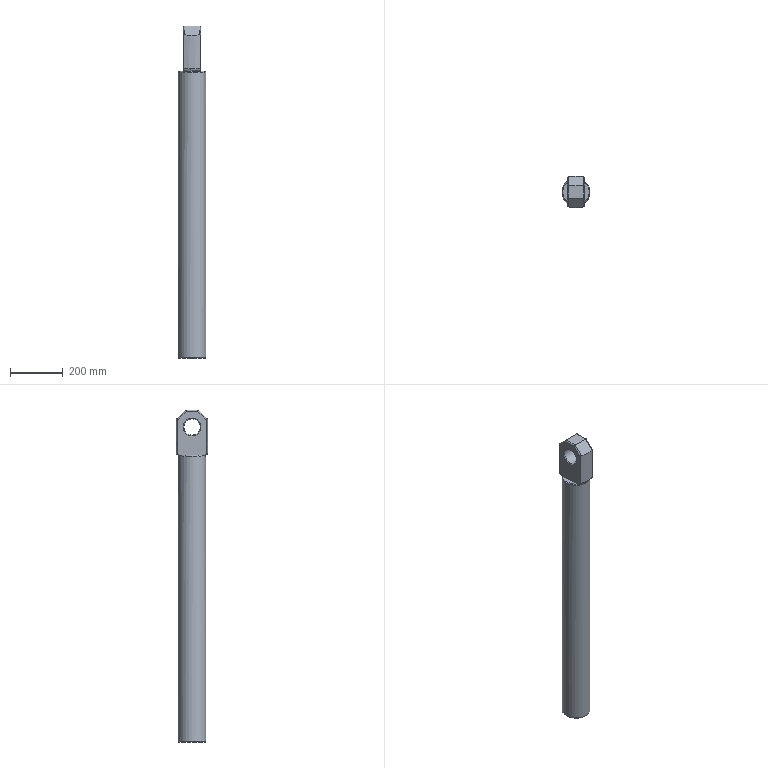Part | NX | features 推移千斤顶活塞 2 | 1 solid | 26 faces | box 106.3 x 120.47 x 1261 mm | volume 10694769 mm3 | cylinder 10 | plane 10 | cone 4 | torus 2 | commonest cylinder face diameters 10 x6 240.94 x2 62 x1 106.3 x1
STEP:
#1=CARTESIAN_POINT('',(-32.42,55.791,1222.469));
#2=VERTEX_POINT('',#1);
#3=CARTESIAN_POINT('',(-32.42,55.791,1099.14));
#4=VERTEX_POINT('',#3);
#5=CARTESIAN_POINT('',(-32.42,55.791,1261.34));
#6=DIRECTION('',(0.,0.,-1.));
#7=VECTOR('',#6,1000.);
#8=LINE('',#5,#7);
#9=EDGE_CURVE('',#2,#4,#8,.T.);
#10=ORIENTED_EDGE('',*,*,#9,.F.);
#11=CARTESIAN_POINT('',(-27.42,57.073,1228.257));
#12=VERTEX_POINT('',#11);
#13=CARTESIAN_POINT('',(-32.42,55.791,1222.469));
#14=CARTESIAN_POINT('',(-32.42,55.791,1223.22));
#15=CARTESIAN_POINT('',(-32.256,55.837,1224.702));
#16=CARTESIAN_POINT('',(-31.381,56.079,1226.805));
#17=CARTESIAN_POINT('',(-29.666,56.532,1228.32));
#18=CARTESIAN_POINT('',(-28.139,56.905,1228.425));
#19=CARTESIAN_POINT('',(-27.42,57.073,1228.257));
#20=B_SPLINE_CURVE_WITH_KNOTS('',3,(#13,#14,#15,#16,#17,#18,#19),.UNSPECIFIED.,.F.,.F.,(4,1,1,1,4),(0.,0.002231,0.004461,0.006692,0.008922),.UNSPECIFIED.);
#21=EDGE_CURVE('',#2,#12,#20,.T.);
#22=ORIENTED_EDGE('',*,*,#21,.T.);
#23=CARTESIAN_POINT('',(27.42,57.073,1228.257));
#24=VERTEX_POINT('',#23);
#25=CARTESIAN_POINT('',(0.,-60.235,1345.565));
#26=DIRECTION('',(0.,0.7071,0.7071));
#27=DIRECTION('',(0.,0.7071,-0.7071));
#28=AXIS2_PLACEMENT_3D('',#25,#26,#27);
#29=ELLIPSE('',#28,170.37,120.47);
#30=EDGE_CURVE('',#24,#12,#29,.T.);
#31=ORIENTED_EDGE('',*,*,#30,.F.);
#32=CARTESIAN_POINT('',(32.42,55.791,1222.469));
#33=VERTEX_POINT('',#32);
#34=CARTESIAN_POINT('',(27.42,57.073,1228.257));
#35=CARTESIAN_POINT('',(28.138,56.905,1228.425));
#36=CARTESIAN_POINT('',(29.654,56.535,1228.326));
#37=CARTESIAN_POINT('',(31.384,56.078,1226.8));
#38=CARTESIAN_POINT('',(32.251,55.838,1224.718));
#39=CARTESIAN_POINT('',(32.42,55.791,1223.22));
#40=CARTESIAN_POINT('',(32.42,55.791,1222.469));
#41=B_SPLINE_CURVE_WITH_KNOTS('',3,(#34,#35,#36,#37,#38,#39,#40),.UNSPECIFIED.,.F.,.F.,(4,1,1,1,4),(0.,0.002239,0.004478,0.006717,0.008957),.UNSPECIFIED.);
#42=EDGE_CURVE('',#24,#33,#41,.T.);
#43=ORIENTED_EDGE('',*,*,#42,.T.);
#44=CARTESIAN_POINT('',(32.42,55.791,1099.14));
#45=VERTEX_POINT('',#44);
#46=CARTESIAN_POINT('',(32.42,55.791,1261.34));
#47=DIRECTION('',(0.,0.,-1.));
#48=VECTOR('',#47,1000.);
#49=LINE('',#46,#48);
#50=EDGE_CURVE('',#33,#45,#49,.T.);
#51=ORIENTED_EDGE('',*,*,#50,.T.);
#52=CARTESIAN_POINT('',(0.,-60.235,1099.14));
#53=DIRECTION('',(0.,0.,1.));
#54=DIRECTION('',(1.,0.,0.));
#55=AXIS2_PLACEMENT_3D('',#52,#53,#54);
#56=CIRCLE('',#55,120.47);
#57=EDGE_CURVE('',#45,#4,#56,.T.);
#58=ORIENTED_EDGE('',*,*,#57,.T.);
#59=EDGE_LOOP('',(#10,#22,#31,#43,#51,#58));
#60=FACE_BOUND('',#59,.T.);
#61=CARTESIAN_POINT('',(0.,-60.235,1261.34));
#62=DIRECTION('',(0.,0.,-1.));
#63=DIRECTION('',(-1.,0.,0.));
#64=AXIS2_PLACEMENT_3D('',#61,#62,#63);
#65=CYLINDRICAL_SURFACE('',#64,120.47);
#66=ADVANCED_FACE('',(#60),#65,.T.);
#67=CARTESIAN_POINT('',(-32.42,34.,1196.49));
#68=VERTEX_POINT('',#67);
#69=CARTESIAN_POINT('',(-32.42,0.,1196.49));
#70=DIRECTION('',(1.,0.,0.));
#71=DIRECTION('',(0.,1.,0.));
#72=AXIS2_PLACEMENT_3D('',#69,#70,#71);
#73=CIRCLE('',#72,34.);
#74=EDGE_CURVE('',#68,#68,#73,.T.);
#75=ORIENTED_EDGE('',*,*,#74,.T.);
#76=EDGE_LOOP('',(#75));
#77=FACE_BOUND('',#76,.T.);
#78=CARTESIAN_POINT('',(-32.42,-21.919,1256.34));
#79=VERTEX_POINT('',#78);
#80=CARTESIAN_POINT('',(-32.42,21.919,1256.34));
#81=VERTEX_POINT('',#80);
#82=CARTESIAN_POINT('',(-32.42,23.99,1256.34));
#83=DIRECTION('',(0.,-1.,0.));
#84=VECTOR('',#83,1000.);
#85=LINE('',#82,#84);
#86=EDGE_CURVE('',#79,#81,#85,.F.);
#87=ORIENTED_EDGE('',*,*,#86,.T.);
#88=CARTESIAN_POINT('',(-32.42,52.255,1226.004));
#89=DIRECTION('',(0.,-0.7071,0.7071));
#90=VECTOR('',#89,1000.);
#91=LINE('',#88,#90);
#92=EDGE_CURVE('',#81,#2,#91,.F.);
#93=ORIENTED_EDGE('',*,*,#92,.T.);
#94=ORIENTED_EDGE('',*,*,#9,.T.);
#95=CARTESIAN_POINT('',(-32.42,45.371,1089.14));
#96=VERTEX_POINT('',#95);
#97=CARTESIAN_POINT('',(-32.42,55.791,1099.14));
#98=CARTESIAN_POINT('',(-32.42,55.791,1096.442));
#99=CARTESIAN_POINT('',(-32.42,53.409,1091.199));
#100=CARTESIAN_POINT('',(-32.42,48.066,1089.14));
#101=CARTESIAN_POINT('',(-32.42,45.371,1089.14));
#102=B_SPLINE_CURVE_WITH_KNOTS('',3,(#97,#98,#99,#100,#101),.UNSPECIFIED.,.F.,.F.,(4,1,4),(0.,0.007978,0.01596),.UNSPECIFIED.);
#103=EDGE_CURVE('',#4,#96,#102,.T.);
#104=ORIENTED_EDGE('',*,*,#103,.T.);
#105=CARTESIAN_POINT('',(-32.42,38.262,1089.14));
#106=VERTEX_POINT('',#105);
#107=CARTESIAN_POINT('',(-32.42,55.791,1089.14));
#108=DIRECTION('',(0.,-1.,0.));
#109=VECTOR('',#108,1000.);
#110=LINE('',#107,#109);
#111=EDGE_CURVE('',#96,#106,#110,.T.);
#112=ORIENTED_EDGE('',*,*,#111,.T.);
#113=CARTESIAN_POINT('',(-32.42,-38.262,1089.14));
#114=VERTEX_POINT('',#113);
#115=CARTESIAN_POINT('',(-32.42,55.791,1089.14));
#116=DIRECTION('',(0.,-1.,0.));
#117=VECTOR('',#116,1000.);
#118=LINE('',#115,#117);
#119=EDGE_CURVE('',#106,#114,#118,.T.);
#120=ORIENTED_EDGE('',*,*,#119,.T.);
#121=CARTESIAN_POINT('',(-32.42,-45.371,1089.14));
#122=VERTEX_POINT('',#121);
#123=CARTESIAN_POINT('',(-32.42,55.791,1089.14));
#124=DIRECTION('',(0.,-1.,0.));
#125=VECTOR('',#124,1000.);
#126=LINE('',#123,#125);
#127=EDGE_CURVE('',#114,#122,#126,.T.);
#128=ORIENTED_EDGE('',*,*,#127,.T.);
#129=CARTESIAN_POINT('',(-32.42,-55.791,1099.14));
#130=VERTEX_POINT('',#129);
#131=CARTESIAN_POINT('',(-32.42,-45.371,1089.14));
#132=CARTESIAN_POINT('',(-32.42,-48.068,1089.14));
#133=CARTESIAN_POINT('',(-32.42,-53.397,1091.189));
#134=CARTESIAN_POINT('',(-32.42,-55.791,1096.44));
#135=CARTESIAN_POINT('',(-32.42,-55.791,1099.14));
#136=B_SPLINE_CURVE_WITH_KNOTS('',3,(#131,#132,#133,#134,#135),.UNSPECIFIED.,.F.,.F.,(4,1,4),(0.,0.007978,0.01596),.UNSPECIFIED.);
#137=EDGE_CURVE('',#122,#130,#136,.T.);
#138=ORIENTED_EDGE('',*,*,#137,.T.);
#139=CARTESIAN_POINT('',(-32.42,-55.791,1222.469));
#140=VERTEX_POINT('',#139);
#141=CARTESIAN_POINT('',(-32.42,-55.791,1261.34));
#142=DIRECTION('',(0.,0.,-1.));
#143=VECTOR('',#142,1000.);
#144=LINE('',#141,#143);
#145=EDGE_CURVE('',#140,#130,#144,.T.);
#146=ORIENTED_EDGE('',*,*,#145,.F.);
#147=CARTESIAN_POINT('',(-32.42,-20.455,1257.804));
#148=DIRECTION('',(0.,-0.7071,-0.7071));
#149=VECTOR('',#148,1000.);
#150=LINE('',#147,#149);
#151=EDGE_CURVE('',#140,#79,#150,.F.);
#152=ORIENTED_EDGE('',*,*,#151,.T.);
#153=EDGE_LOOP('',(#87,#93,#94,#104,#112,#120,#128,#138,#146,#152));
#154=FACE_BOUND('',#153,.T.);
#155=CARTESIAN_POINT('',(-32.42,55.791,1261.34));
#156=DIRECTION('',(1.,0.,0.));
#157=DIRECTION('',(0.,1.,0.));
#158=AXIS2_PLACEMENT_3D('',#155,#156,#157);
#159=PLANE('',#158);
#160=ADVANCED_FACE('',(#77,#154),#159,.F.);
#161=CARTESIAN_POINT('',(-27.42,-57.073,1228.257));
#162=VERTEX_POINT('',#161);
#163=CARTESIAN_POINT('',(27.42,-57.073,1228.257));
#164=VERTEX_POINT('',#163);
#165=CARTESIAN_POINT('',(0.,60.235,1345.565));
#166=DIRECTION('',(0.,-0.7071,0.7071));
#167=DIRECTION('',(0.,-0.7071,-0.7071));
#168=AXIS2_PLACEMENT_3D('',#165,#166,#167);
#169=ELLIPSE('',#168,170.37,120.47);
#170=EDGE_CURVE('',#162,#164,#169,.T.);
#171=ORIENTED_EDGE('',*,*,#170,.F.);
#172=CARTESIAN_POINT('',(-27.42,-57.073,1228.257));
#173=CARTESIAN_POINT('',(-28.138,-56.905,1228.425));
#174=CARTESIAN_POINT('',(-29.654,-56.535,1228.326));
#175=CARTESIAN_POINT('',(-31.384,-56.078,1226.8));
#176=CARTESIAN_POINT('',(-32.251,-55.838,1224.718));
#177=CARTESIAN_POINT('',(-32.42,-55.791,1223.22));
#178=CARTESIAN_POINT('',(-32.42,-55.791,1222.469));
#179=B_SPLINE_CURVE_WITH_KNOTS('',3,(#172,#173,#174,#175,#176,#177,#178),.UNSPECIFIED.,.F.,.F.,(4,1,1,1,4),(0.,0.002239,0.004478,0.006717,0.008957),.UNSPECIFIED.);
#180=EDGE_CURVE('',#162,#140,#179,.T.);
#181=ORIENTED_EDGE('',*,*,#180,.T.);
#182=ORIENTED_EDGE('',*,*,#145,.T.);
#183=CARTESIAN_POINT('',(32.42,-55.791,1099.14));
#184=VERTEX_POINT('',#183);
#185=CARTESIAN_POINT('',(0.,60.235,1099.14));
#186=DIRECTION('',(0.,0.,1.));
#187=DIRECTION('',(1.,0.,0.));
#188=AXIS2_PLACEMENT_3D('',#185,#186,#187);
#189=CIRCLE('',#188,120.47);
#190=EDGE_CURVE('',#130,#184,#189,.T.);
#191=ORIENTED_EDGE('',*,*,#190,.T.);
#192=CARTESIAN_POINT('',(32.42,-55.791,1222.469));
#193=VERTEX_POINT('',#192);
#194=CARTESIAN_POINT('',(32.42,-55.791,1261.34));
#195=DIRECTION('',(0.,0.,-1.));
#196=VECTOR('',#195,1000.);
#197=LINE('',#194,#196);
#198=EDGE_CURVE('',#193,#184,#197,.T.);
#199=ORIENTED_EDGE('',*,*,#198,.F.);
#200=CARTESIAN_POINT('',(32.42,-55.791,1222.469));
#201=CARTESIAN_POINT('',(32.42,-55.791,1223.22));
#202=CARTESIAN_POINT('',(32.256,-55.837,1224.702));
#203=CARTESIAN_POINT('',(31.381,-56.079,1226.805));
#204=CARTESIAN_POINT('',(29.666,-56.532,1228.32));
#205=CARTESIAN_POINT('',(28.139,-56.905,1228.425));
#206=CARTESIAN_POINT('',(27.42,-57.073,1228.257));
#207=B_SPLINE_CURVE_WITH_KNOTS('',3,(#200,#201,#202,#203,#204,#205,#206),.UNSPECIFIED.,.F.,.F.,(4,1,1,1,4),(0.,0.002231,0.004461,0.006692,0.008922),.UNSPECIFIED.);
#208=EDGE_CURVE('',#193,#164,#207,.T.);
#209=ORIENTED_EDGE('',*,*,#208,.T.);
#210=EDGE_LOOP('',(#171,#181,#182,#191,#199,#209));
#211=FACE_BOUND('',#210,.T.);
#212=CARTESIAN_POINT('',(0.,60.235,1261.34));
#213=DIRECTION('',(0.,0.,-1.));
#214=DIRECTION('',(-1.,0.,0.));
#215=AXIS2_PLACEMENT_3D('',#212,#213,#214);
#216=CYLINDRICAL_SURFACE('',#215,120.47);
#217=ADVANCED_FACE('',(#211),#216,.T.);
#218=CARTESIAN_POINT('',(32.42,0.,1230.49));
#219=VERTEX_POINT('',#218);
#220=CARTESIAN_POINT('',(32.42,0.,1196.49));
#221=DIRECTION('',(-1.,0.,0.));
#222=DIRECTION('',(0.,0.,1.));
#223=AXIS2_PLACEMENT_3D('',#220,#221,#222);
#224=CIRCLE('',#223,34.);
#225=EDGE_CURVE('',#219,#219,#224,.T.);
#226=ORIENTED_EDGE('',*,*,#225,.T.);
#227=EDGE_LOOP('',(#226));
#228=FACE_BOUND('',#227,.T.);
#229=CARTESIAN_POINT('',(32.42,21.919,1256.34));
#230=VERTEX_POINT('',#229);
#231=CARTESIAN_POINT('',(32.42,-21.919,1256.34));
#232=VERTEX_POINT('',#231);
#233=CARTESIAN_POINT('',(32.42,-23.99,1256.34));
#234=DIRECTION('',(0.,1.,0.));
#235=VECTOR('',#234,1000.);
#236=LINE('',#233,#235);
#237=EDGE_CURVE('',#230,#232,#236,.F.);
#238=ORIENTED_EDGE('',*,*,#237,.T.);
#239=CARTESIAN_POINT('',(32.42,-52.255,1226.004));
#240=DIRECTION('',(0.,0.7071,0.7071));
#241=VECTOR('',#240,1000.);
#242=LINE('',#239,#241);
#243=EDGE_CURVE('',#232,#193,#242,.F.);
#244=ORIENTED_EDGE('',*,*,#243,.T.);
#245=ORIENTED_EDGE('',*,*,#198,.T.);
#246=CARTESIAN_POINT('',(32.42,-45.371,1089.14));
#247=VERTEX_POINT('',#246);
#248=CARTESIAN_POINT('',(32.42,-55.791,1099.14));
#249=CARTESIAN_POINT('',(32.42,-55.791,1096.442));
#250=CARTESIAN_POINT('',(32.42,-53.409,1091.199));
#251=CARTESIAN_POINT('',(32.42,-48.066,1089.14));
#252=CARTESIAN_POINT('',(32.42,-45.371,1089.14));
#253=B_SPLINE_CURVE_WITH_KNOTS('',3,(#248,#249,#250,#251,#252),.UNSPECIFIED.,.F.,.F.,(4,1,4),(0.,0.007978,0.01596),.UNSPECIFIED.);
#254=EDGE_CURVE('',#184,#247,#253,.T.);
#255=ORIENTED_EDGE('',*,*,#254,.T.);
#256=CARTESIAN_POINT('',(32.42,-38.262,1089.14));
#257=VERTEX_POINT('',#256);
#258=CARTESIAN_POINT('',(32.42,55.791,1089.14));
#259=DIRECTION('',(0.,1.,0.));
#260=VECTOR('',#259,1000.);
#261=LINE('',#258,#260);
#262=EDGE_CURVE('',#247,#257,#261,.T.);
#263=ORIENTED_EDGE('',*,*,#262,.T.);
#264=CARTESIAN_POINT('',(32.42,38.262,1089.14));
#265=VERTEX_POINT('',#264);
#266=CARTESIAN_POINT('',(32.42,55.791,1089.14));
#267=DIRECTION('',(0.,1.,0.));
#268=VECTOR('',#267,1000.);
#269=LINE('',#266,#268);
#270=EDGE_CURVE('',#257,#265,#269,.T.);
#271=ORIENTED_EDGE('',*,*,#270,.T.);
#272=CARTESIAN_POINT('',(32.42,45.371,1089.14));
#273=VERTEX_POINT('',#272);
#274=CARTESIAN_POINT('',(32.42,55.791,1089.14));
#275=DIRECTION('',(0.,1.,0.));
#276=VECTOR('',#275,1000.);
#277=LINE('',#274,#276);
#278=EDGE_CURVE('',#265,#273,#277,.T.);
#279=ORIENTED_EDGE('',*,*,#278,.T.);
#280=CARTESIAN_POINT('',(32.42,45.371,1089.14));
#281=CARTESIAN_POINT('',(32.42,48.068,1089.14));
#282=CARTESIAN_POINT('',(32.42,53.397,1091.189));
#283=CARTESIAN_POINT('',(32.42,55.791,1096.44));
#284=CARTESIAN_POINT('',(32.42,55.791,1099.14));
#285=B_SPLINE_CURVE_WITH_KNOTS('',3,(#280,#281,#282,#283,#284),.UNSPECIFIED.,.F.,.F.,(4,1,4),(0.,0.007978,0.01596),.UNSPECIFIED.);
#286=EDGE_CURVE('',#273,#45,#285,.T.);
#287=ORIENTED_EDGE('',*,*,#286,.T.);
#288=ORIENTED_EDGE('',*,*,#50,.F.);
#289=CARTESIAN_POINT('',(32.42,20.455,1257.804));
#290=DIRECTION('',(0.,0.7071,-0.7071));
#291=VECTOR('',#290,1000.);
#292=LINE('',#289,#291);
#293=EDGE_CURVE('',#33,#230,#292,.F.);
#294=ORIENTED_EDGE('',*,*,#293,.T.);
#295=EDGE_LOOP('',(#238,#244,#245,#255,#263,#271,#279,#287,#288,#294));
#296=FACE_BOUND('',#295,.T.);
#297=CARTESIAN_POINT('',(32.42,55.791,1261.34));
#298=DIRECTION('',(-1.,0.,0.));
#299=DIRECTION('',(0.,0.,1.));
#300=AXIS2_PLACEMENT_3D('',#297,#298,#299);
#301=PLANE('',#300);
#302=ADVANCED_FACE('',(#228,#296),#301,.F.);
#303=CARTESIAN_POINT('',(27.42,23.99,1261.34));
#304=VERTEX_POINT('',#303);
#305=CARTESIAN_POINT('',(-27.42,23.99,1261.34));
#306=VERTEX_POINT('',#305);
#307=CARTESIAN_POINT('',(1621.834,23.99,1261.34));
#308=DIRECTION('',(-1.,0.,0.));
#309=VECTOR('',#308,1000.);
#310=LINE('',#307,#309);
#311=EDGE_CURVE('',#304,#306,#310,.T.);
#312=ORIENTED_EDGE('',*,*,#311,.T.);
#313=CARTESIAN_POINT('',(-27.42,-23.99,1261.34));
#314=VERTEX_POINT('',#313);
#315=CARTESIAN_POINT('',(-27.42,-23.99,1261.34));
#316=DIRECTION('',(0.,-1.,0.));
#317=VECTOR('',#316,1000.);
#318=LINE('',#315,#317);
#319=EDGE_CURVE('',#306,#314,#318,.T.);
#320=ORIENTED_EDGE('',*,*,#319,.T.);
#321=CARTESIAN_POINT('',(27.42,-23.99,1261.34));
#322=VERTEX_POINT('',#321);
#323=CARTESIAN_POINT('',(0.,-23.99,1261.34));
#324=DIRECTION('',(1.,0.,0.));
#325=VECTOR('',#324,1000.);
#326=LINE('',#323,#325);
#327=EDGE_CURVE('',#314,#322,#326,.T.);
#328=ORIENTED_EDGE('',*,*,#327,.T.);
#329=CARTESIAN_POINT('',(27.42,23.99,1261.34));
#330=DIRECTION('',(0.,1.,0.));
#331=VECTOR('',#330,1000.);
#332=LINE('',#329,#331);
#333=EDGE_CURVE('',#322,#304,#332,.T.);
#334=ORIENTED_EDGE('',*,*,#333,.T.);
#335=EDGE_LOOP('',(#312,#320,#328,#334));
#336=FACE_BOUND('',#335,.T.);
#337=CARTESIAN_POINT('',(0.,-60.235,1261.34));
#338=DIRECTION('',(0.,0.,1.));
#339=DIRECTION('',(1.,0.,0.));
#340=AXIS2_PLACEMENT_3D('',#337,#338,#339);
#341=PLANE('',#340);
#342=ADVANCED_FACE('',(#336),#341,.T.);
#343=ORIENTED_EDGE('',*,*,#270,.F.);
#344=CARTESIAN_POINT('',(0.,0.,1089.14));
#345=DIRECTION('',(0.,0.,1.));
#346=DIRECTION('',(1.,0.,0.));
#347=AXIS2_PLACEMENT_3D('',#344,#345,#346);
#348=CIRCLE('',#347,50.15);
#349=EDGE_CURVE('',#257,#265,#348,.T.);
#350=ORIENTED_EDGE('',*,*,#349,.T.);
#351=EDGE_LOOP('',(#343,#350));
#352=FACE_BOUND('',#351,.T.);
#353=CARTESIAN_POINT('',(0.,0.,1089.14));
#354=DIRECTION('',(0.,0.,1.));
#355=DIRECTION('',(1.,0.,0.));
#356=AXIS2_PLACEMENT_3D('',#353,#354,#355);
#357=PLANE('',#356);
#358=ADVANCED_FACE('',(#352),#357,.T.);
#359=CARTESIAN_POINT('',(53.15,0.,1086.14));
#360=VERTEX_POINT('',#359);
#361=CARTESIAN_POINT('',(0.,0.,1086.14));
#362=DIRECTION('',(0.,0.,1.));
#363=DIRECTION('',(1.,0.,0.));
#364=AXIS2_PLACEMENT_3D('',#361,#362,#363);
#365=CIRCLE('',#364,53.15);
#366=EDGE_CURVE('',#360,#360,#365,.F.);
#367=ORIENTED_EDGE('',*,*,#366,.T.);
#368=EDGE_LOOP('',(#367));
#369=FACE_BOUND('',#368,.T.);
#370=CARTESIAN_POINT('',(53.15,0.,3.));
#371=VERTEX_POINT('',#370);
#372=CARTESIAN_POINT('',(0.,0.,3.));
#373=DIRECTION('',(0.,0.,1.));
#374=DIRECTION('',(1.,0.,0.));
#375=AXIS2_PLACEMENT_3D('',#372,#373,#374);
#376=CIRCLE('',#375,53.15);
#377=EDGE_CURVE('',#371,#371,#376,.T.);
#378=ORIENTED_EDGE('',*,*,#377,.T.);
#379=EDGE_LOOP('',(#378));
#380=FACE_BOUND('',#379,.T.);
#381=CARTESIAN_POINT('',(0.,0.,1089.14));
#382=DIRECTION('',(0.,0.,-1.));
#383=DIRECTION('',(-1.,0.,0.));
#384=AXIS2_PLACEMENT_3D('',#381,#382,#383);
#385=CYLINDRICAL_SURFACE('',#384,53.15);
#386=ADVANCED_FACE('',(#369,#380),#385,.T.);
#387=ORIENTED_EDGE('',*,*,#119,.F.);
#388=CARTESIAN_POINT('',(0.,0.,1089.14));
#389=DIRECTION('',(0.,0.,1.));
#390=DIRECTION('',(1.,0.,0.));
#391=AXIS2_PLACEMENT_3D('',#388,#389,#390);
#392=CIRCLE('',#391,50.15);
#393=EDGE_CURVE('',#106,#114,#392,.T.);
#394=ORIENTED_EDGE('',*,*,#393,.T.);
#395=EDGE_LOOP('',(#387,#394));
#396=FACE_BOUND('',#395,.T.);
#397=CARTESIAN_POINT('',(0.,0.,1089.14));
#398=DIRECTION('',(0.,0.,1.));
#399=DIRECTION('',(1.,0.,0.));
#400=AXIS2_PLACEMENT_3D('',#397,#398,#399);
#401=PLANE('',#400);
#402=ADVANCED_FACE('',(#396),#401,.T.);
#403=CARTESIAN_POINT('',(50.15,0.,0.));
#404=VERTEX_POINT('',#403);
#405=CARTESIAN_POINT('',(0.,0.,0.));
#406=DIRECTION('',(0.,0.,1.));
#407=DIRECTION('',(1.,0.,0.));
#408=AXIS2_PLACEMENT_3D('',#405,#406,#407);
#409=CIRCLE('',#408,50.15);
#410=EDGE_CURVE('',#404,#404,#409,.F.);
#411=ORIENTED_EDGE('',*,*,#410,.T.);
#412=EDGE_LOOP('',(#411));
#413=FACE_BOUND('',#412,.T.);
#414=CARTESIAN_POINT('',(0.,0.,0.));
#415=DIRECTION('',(0.,0.,1.));
#416=DIRECTION('',(1.,0.,0.));
#417=AXIS2_PLACEMENT_3D('',#414,#415,#416);
#418=PLANE('',#417);
#419=ADVANCED_FACE('',(#413),#418,.F.);
#420=ORIENTED_EDGE('',*,*,#366,.F.);
#421=EDGE_LOOP('',(#420));
#422=FACE_BOUND('',#421,.T.);
#423=CARTESIAN_POINT('',(0.,0.,1089.14));
#424=DIRECTION('',(0.,0.,1.));
#425=DIRECTION('',(1.,0.,0.));
#426=AXIS2_PLACEMENT_3D('',#423,#424,#425);
#427=CIRCLE('',#426,50.15);
#428=EDGE_CURVE('',#265,#106,#427,.T.);
#429=ORIENTED_EDGE('',*,*,#428,.F.);
#430=ORIENTED_EDGE('',*,*,#349,.F.);
#431=CARTESIAN_POINT('',(0.,0.,1089.14));
#432=DIRECTION('',(0.,0.,1.));
#433=DIRECTION('',(1.,0.,0.));
#434=AXIS2_PLACEMENT_3D('',#431,#432,#433);
#435=CIRCLE('',#434,50.15);
#436=EDGE_CURVE('',#114,#257,#435,.T.);
#437=ORIENTED_EDGE('',*,*,#436,.F.);
#438=ORIENTED_EDGE('',*,*,#393,.F.);
#439=EDGE_LOOP('',(#429,#430,#437,#438));
#440=FACE_BOUND('',#439,.T.);
#441=CARTESIAN_POINT('',(0.,0.,1089.14));
#442=DIRECTION('',(0.,0.,-1.));
#443=DIRECTION('',(-1.,0.,0.));
#444=AXIS2_PLACEMENT_3D('',#441,#442,#443);
#445=CONICAL_SURFACE('',#444,50.15,0.7854);
#446=ADVANCED_FACE('',(#422,#440),#445,.T.);
#447=ORIENTED_EDGE('',*,*,#410,.F.);
#448=EDGE_LOOP('',(#447));
#449=FACE_BOUND('',#448,.T.);
#450=ORIENTED_EDGE('',*,*,#377,.F.);
#451=EDGE_LOOP('',(#450));
#452=FACE_BOUND('',#451,.T.);
#453=CARTESIAN_POINT('',(0.,0.,3.));
#454=DIRECTION('',(0.,0.,1.));
#455=DIRECTION('',(1.,0.,0.));
#456=AXIS2_PLACEMENT_3D('',#453,#454,#455);
#457=CONICAL_SURFACE('',#456,53.15,0.7854);
#458=ADVANCED_FACE('',(#449,#452),#457,.T.);
#459=ORIENTED_EDGE('',*,*,#111,.F.);
#460=CARTESIAN_POINT('',(0.,-60.235,1089.14));
#461=DIRECTION('',(0.,0.,1.));
#462=DIRECTION('',(1.,0.,0.));
#463=AXIS2_PLACEMENT_3D('',#460,#461,#462);
#464=CIRCLE('',#463,110.47);
#465=EDGE_CURVE('',#96,#273,#464,.F.);
#466=ORIENTED_EDGE('',*,*,#465,.T.);
#467=ORIENTED_EDGE('',*,*,#278,.F.);
#468=ORIENTED_EDGE('',*,*,#428,.T.);
#469=EDGE_LOOP('',(#459,#466,#467,#468));
#470=FACE_BOUND('',#469,.T.);
#471=CARTESIAN_POINT('',(0.,-60.235,1089.14));
#472=DIRECTION('',(0.,0.,1.));
#473=DIRECTION('',(1.,0.,0.));
#474=AXIS2_PLACEMENT_3D('',#471,#472,#473);
#475=PLANE('',#474);
#476=ADVANCED_FACE('',(#470),#475,.F.);
#477=ORIENTED_EDGE('',*,*,#262,.F.);
#478=CARTESIAN_POINT('',(0.,60.235,1089.14));
#479=DIRECTION('',(0.,0.,1.));
#480=DIRECTION('',(1.,0.,0.));
#481=AXIS2_PLACEMENT_3D('',#478,#479,#480);
#482=CIRCLE('',#481,110.47);
#483=EDGE_CURVE('',#247,#122,#482,.F.);
#484=ORIENTED_EDGE('',*,*,#483,.T.);
#485=ORIENTED_EDGE('',*,*,#127,.F.);
#486=ORIENTED_EDGE('',*,*,#436,.T.);
#487=EDGE_LOOP('',(#477,#484,#485,#486));
#488=FACE_BOUND('',#487,.T.);
#489=CARTESIAN_POINT('',(0.,-60.235,1089.14));
#490=DIRECTION('',(0.,0.,1.));
#491=DIRECTION('',(1.,0.,0.));
#492=AXIS2_PLACEMENT_3D('',#489,#490,#491);
#493=PLANE('',#492);
#494=ADVANCED_FACE('',(#488),#493,.F.);
#495=ORIENTED_EDGE('',*,*,#137,.F.);
#496=ORIENTED_EDGE('',*,*,#483,.F.);
#497=ORIENTED_EDGE('',*,*,#254,.F.);
#498=ORIENTED_EDGE('',*,*,#190,.F.);
#499=EDGE_LOOP('',(#495,#496,#497,#498));
#500=FACE_BOUND('',#499,.T.);
#501=CARTESIAN_POINT('',(0.,60.235,1099.14));
#502=DIRECTION('',(0.,0.,1.));
#503=DIRECTION('',(1.,0.,0.));
#504=AXIS2_PLACEMENT_3D('',#501,#502,#503);
#505=TOROIDAL_SURFACE('',#504,110.47,10.);
#506=ADVANCED_FACE('',(#500),#505,.T.);
#507=ORIENTED_EDGE('',*,*,#286,.F.);
#508=ORIENTED_EDGE('',*,*,#465,.F.);
#509=ORIENTED_EDGE('',*,*,#103,.F.);
#510=ORIENTED_EDGE('',*,*,#57,.F.);
#511=EDGE_LOOP('',(#507,#508,#509,#510));
#512=FACE_BOUND('',#511,.T.);
#513=CARTESIAN_POINT('',(0.,-60.235,1099.14));
#514=DIRECTION('',(0.,0.,1.));
#515=DIRECTION('',(1.,0.,0.));
#516=AXIS2_PLACEMENT_3D('',#513,#514,#515);
#517=TOROIDAL_SURFACE('',#516,110.47,10.);
#518=ADVANCED_FACE('',(#512),#517,.T.);
#519=CARTESIAN_POINT('',(-29.42,0.,1165.49));
#520=VERTEX_POINT('',#519);
#521=CARTESIAN_POINT('',(-29.42,0.,1196.49));
#522=DIRECTION('',(1.,0.,0.));
#523=DIRECTION('',(0.,0.,-1.));
#524=AXIS2_PLACEMENT_3D('',#521,#522,#523);
#525=CIRCLE('',#524,31.);
#526=EDGE_CURVE('',#520,#520,#525,.F.);
#527=ORIENTED_EDGE('',*,*,#526,.T.);
#528=EDGE_LOOP('',(#527));
#529=FACE_BOUND('',#528,.T.);
#530=CARTESIAN_POINT('',(29.42,0.,1227.49));
#531=VERTEX_POINT('',#530);
#532=CARTESIAN_POINT('',(29.42,0.,1196.49));
#533=DIRECTION('',(-1.,0.,0.));
#534=DIRECTION('',(0.,0.,1.));
#535=AXIS2_PLACEMENT_3D('',#532,#533,#534);
#536=CIRCLE('',#535,31.);
#537=EDGE_CURVE('',#531,#531,#536,.F.);
#538=ORIENTED_EDGE('',*,*,#537,.T.);
#539=EDGE_LOOP('',(#538));
#540=FACE_BOUND('',#539,.T.);
#541=CARTESIAN_POINT('',(-139.78,0.,1196.49));
#542=DIRECTION('',(1.,0.,0.));
#543=DIRECTION('',(0.,0.,-1.));
#544=AXIS2_PLACEMENT_3D('',#541,#542,#543);
#545=CYLINDRICAL_SURFACE('',#544,31.);
#546=ADVANCED_FACE('',(#529,#540),#545,.F.);
#547=ORIENTED_EDGE('',*,*,#526,.F.);
#548=EDGE_LOOP('',(#547));
#549=FACE_BOUND('',#548,.T.);
#550=ORIENTED_EDGE('',*,*,#74,.F.);
#551=EDGE_LOOP('',(#550));
#552=FACE_BOUND('',#551,.T.);
#553=CARTESIAN_POINT('',(-32.42,0.,1196.49));
#554=DIRECTION('',(-1.,0.,0.));
#555=DIRECTION('',(0.,0.,1.));
#556=AXIS2_PLACEMENT_3D('',#553,#554,#555);
#557=CONICAL_SURFACE('',#556,34.,0.7854);
#558=ADVANCED_FACE('',(#549,#552),#557,.F.);
#559=ORIENTED_EDGE('',*,*,#225,.F.);
#560=EDGE_LOOP('',(#559));
#561=FACE_BOUND('',#560,.T.);
#562=ORIENTED_EDGE('',*,*,#537,.F.);
#563=EDGE_LOOP('',(#562));
#564=FACE_BOUND('',#563,.T.);
#565=CARTESIAN_POINT('',(29.42,0.,1196.49));
#566=DIRECTION('',(1.,0.,0.));
#567=DIRECTION('',(0.,0.,-1.));
#568=AXIS2_PLACEMENT_3D('',#565,#566,#567);
#569=CONICAL_SURFACE('',#568,31.,0.7854);
#570=ADVANCED_FACE('',(#561,#564),#569,.F.);
#571=ORIENTED_EDGE('',*,*,#327,.F.);
#572=CARTESIAN_POINT('',(-27.42,-55.791,1229.54));
#573=DIRECTION('',(0.,-0.7071,-0.7071));
#574=VECTOR('',#573,1000.);
#575=LINE('',#572,#574);
#576=EDGE_CURVE('',#314,#162,#575,.T.);
#577=ORIENTED_EDGE('',*,*,#576,.T.);
#578=ORIENTED_EDGE('',*,*,#170,.T.);
#579=CARTESIAN_POINT('',(27.42,-23.99,1261.34));
#580=DIRECTION('',(0.,0.7071,0.7071));
#581=VECTOR('',#580,1000.);
#582=LINE('',#579,#581);
#583=EDGE_CURVE('',#164,#322,#582,.T.);
#584=ORIENTED_EDGE('',*,*,#583,.T.);
#585=EDGE_LOOP('',(#571,#577,#578,#584));
#586=FACE_BOUND('',#585,.T.);
#587=CARTESIAN_POINT('',(1621.834,-65.259,1220.072));
#588=DIRECTION('',(0.,-0.7071,0.7071));
#589=DIRECTION('',(0.,-0.7071,-0.7071));
#590=AXIS2_PLACEMENT_3D('',#587,#588,#589);
#591=PLANE('',#590);
#592=ADVANCED_FACE('',(#586),#591,.T.);
#593=ORIENTED_EDGE('',*,*,#30,.T.);
#594=CARTESIAN_POINT('',(-27.42,23.99,1261.34));
#595=DIRECTION('',(0.,-0.7071,0.7071));
#596=VECTOR('',#595,1000.);
#597=LINE('',#594,#596);
#598=EDGE_CURVE('',#12,#306,#597,.T.);
#599=ORIENTED_EDGE('',*,*,#598,.T.);
#600=ORIENTED_EDGE('',*,*,#311,.F.);
#601=CARTESIAN_POINT('',(27.42,55.791,1229.54));
#602=DIRECTION('',(0.,0.7071,-0.7071));
#603=VECTOR('',#602,1000.);
#604=LINE('',#601,#603);
#605=EDGE_CURVE('',#304,#24,#604,.T.);
#606=ORIENTED_EDGE('',*,*,#605,.T.);
#607=EDGE_LOOP('',(#593,#599,#600,#606));
#608=FACE_BOUND('',#607,.T.);
#609=CARTESIAN_POINT('',(1621.834,65.707,1219.623));
#610=DIRECTION('',(0.,0.7071,0.7071));
#611=DIRECTION('',(0.,-0.7071,0.7071));
#612=AXIS2_PLACEMENT_3D('',#609,#610,#611);
#613=PLANE('',#612);
#614=ADVANCED_FACE('',(#608),#613,.T.);
#615=ORIENTED_EDGE('',*,*,#180,.F.);
#616=ORIENTED_EDGE('',*,*,#576,.F.);
#617=CARTESIAN_POINT('',(-27.42,-21.919,1256.34));
#618=DIRECTION('',(0.,0.9239,0.3827));
#619=DIRECTION('',(0.,-0.3827,0.9239));
#620=AXIS2_PLACEMENT_3D('',#617,#618,#619);
#621=ELLIPSE('',#620,5.412,5.);
#622=EDGE_CURVE('',#79,#314,#621,.T.);
#623=ORIENTED_EDGE('',*,*,#622,.F.);
#624=ORIENTED_EDGE('',*,*,#151,.F.);
#625=EDGE_LOOP('',(#615,#616,#623,#624));
#626=FACE_BOUND('',#625,.T.);
#627=CARTESIAN_POINT('',(-27.42,-61.723,1216.536));
#628=DIRECTION('',(0.,0.7071,0.7071));
#629=DIRECTION('',(0.,-0.7071,0.7071));
#630=AXIS2_PLACEMENT_3D('',#627,#628,#629);
#631=CYLINDRICAL_SURFACE('',#630,5.);
#632=ADVANCED_FACE('',(#626),#631,.T.);
#633=ORIENTED_EDGE('',*,*,#622,.T.);
#634=ORIENTED_EDGE('',*,*,#319,.F.);
#635=CARTESIAN_POINT('',(-27.42,21.919,1256.34));
#636=DIRECTION('',(0.,0.9239,-0.3827));
#637=DIRECTION('',(0.,0.3827,0.9239));
#638=AXIS2_PLACEMENT_3D('',#635,#636,#637);
#639=ELLIPSE('',#638,5.412,5.);
#640=EDGE_CURVE('',#81,#306,#639,.T.);
#641=ORIENTED_EDGE('',*,*,#640,.F.);
#642=ORIENTED_EDGE('',*,*,#86,.F.);
#643=EDGE_LOOP('',(#633,#634,#641,#642));
#644=FACE_BOUND('',#643,.T.);
#645=CARTESIAN_POINT('',(-27.42,-60.235,1256.34));
#646=DIRECTION('',(0.,1.,0.));
#647=DIRECTION('',(-1.,0.,0.));
#648=AXIS2_PLACEMENT_3D('',#645,#646,#647);
#649=CYLINDRICAL_SURFACE('',#648,5.);
#650=ADVANCED_FACE('',(#644),#649,.T.);
#651=ORIENTED_EDGE('',*,*,#21,.F.);
#652=ORIENTED_EDGE('',*,*,#92,.F.);
#653=ORIENTED_EDGE('',*,*,#640,.T.);
#654=ORIENTED_EDGE('',*,*,#598,.F.);
#655=EDGE_LOOP('',(#651,#652,#653,#654));
#656=FACE_BOUND('',#655,.T.);
#657=CARTESIAN_POINT('',(-27.42,62.172,1216.087));
#658=DIRECTION('',(0.,0.7071,-0.7071));
#659=DIRECTION('',(0.,0.7071,0.7071));
#660=AXIS2_PLACEMENT_3D('',#657,#658,#659);
#661=CYLINDRICAL_SURFACE('',#660,5.);
#662=ADVANCED_FACE('',(#656),#661,.T.);
#663=ORIENTED_EDGE('',*,*,#42,.F.);
#664=ORIENTED_EDGE('',*,*,#605,.F.);
#665=CARTESIAN_POINT('',(27.42,21.919,1256.34));
#666=DIRECTION('',(0.,-0.9239,0.3827));
#667=DIRECTION('',(0.,0.3827,0.9239));
#668=AXIS2_PLACEMENT_3D('',#665,#666,#667);
#669=ELLIPSE('',#668,5.412,5.);
#670=EDGE_CURVE('',#230,#304,#669,.T.);
#671=ORIENTED_EDGE('',*,*,#670,.F.);
#672=ORIENTED_EDGE('',*,*,#293,.F.);
#673=EDGE_LOOP('',(#663,#664,#671,#672));
#674=FACE_BOUND('',#673,.T.);
#675=CARTESIAN_POINT('',(27.42,62.172,1216.087));
#676=DIRECTION('',(0.,-0.7071,0.7071));
#677=DIRECTION('',(0.,-0.7071,-0.7071));
#678=AXIS2_PLACEMENT_3D('',#675,#676,#677);
#679=CYLINDRICAL_SURFACE('',#678,5.);
#680=ADVANCED_FACE('',(#674),#679,.T.);
#681=ORIENTED_EDGE('',*,*,#670,.T.);
#682=ORIENTED_EDGE('',*,*,#333,.F.);
#683=CARTESIAN_POINT('',(27.42,-21.919,1256.34));
#684=DIRECTION('',(0.,-0.9239,-0.3827));
#685=DIRECTION('',(0.,-0.3827,0.9239));
#686=AXIS2_PLACEMENT_3D('',#683,#684,#685);
#687=ELLIPSE('',#686,5.412,5.);
#688=EDGE_CURVE('',#232,#322,#687,.T.);
#689=ORIENTED_EDGE('',*,*,#688,.F.);
#690=ORIENTED_EDGE('',*,*,#237,.F.);
#691=EDGE_LOOP('',(#681,#682,#689,#690));
#692=FACE_BOUND('',#691,.T.);
#693=CARTESIAN_POINT('',(27.42,-60.235,1256.34));
#694=DIRECTION('',(0.,-1.,0.));
#695=DIRECTION('',(0.,0.,-1.));
#696=AXIS2_PLACEMENT_3D('',#693,#694,#695);
#697=CYLINDRICAL_SURFACE('',#696,5.);
#698=ADVANCED_FACE('',(#692),#697,.T.);
#699=ORIENTED_EDGE('',*,*,#208,.F.);
#700=ORIENTED_EDGE('',*,*,#243,.F.);
#701=ORIENTED_EDGE('',*,*,#688,.T.);
#702=ORIENTED_EDGE('',*,*,#583,.F.);
#703=EDGE_LOOP('',(#699,#700,#701,#702));
#704=FACE_BOUND('',#703,.T.);
#705=CARTESIAN_POINT('',(27.42,-61.723,1216.536));
#706=DIRECTION('',(0.,-0.7071,-0.7071));
#707=DIRECTION('',(0.,0.7071,-0.7071));
#708=AXIS2_PLACEMENT_3D('',#705,#706,#707);
#709=CYLINDRICAL_SURFACE('',#708,5.);
#710=ADVANCED_FACE('',(#704),#709,.T.);
#711=CLOSED_SHELL('',(#66,#160,#217,#302,#342,#358,#386,#402,#419,#446,#458,#476,#494,#506,#518,#546,#558,#570,#592,#614,#632,#650,#662,#680,#698,#710));
#712=MANIFOLD_SOLID_BREP('',#711);
#713=(LENGTH_UNIT()NAMED_UNIT(*)SI_UNIT(.MILLI.,.METRE.));
#714=UNCERTAINTY_MEASURE_WITH_UNIT(LENGTH_MEASURE(0.0508),#713,'','');
#715=(NAMED_UNIT(*)PLANE_ANGLE_UNIT()SI_UNIT($,.RADIAN.));
#716=(NAMED_UNIT(*)SI_UNIT($,.STERADIAN.)SOLID_ANGLE_UNIT());
#717=(GEOMETRIC_REPRESENTATION_CONTEXT(3)GLOBAL_UNCERTAINTY_ASSIGNED_CONTEXT((#714))GLOBAL_UNIT_ASSIGNED_CONTEXT((#713,#715,#716))REPRESENTATION_CONTEXT('',''));
#718=ADVANCED_BREP_SHAPE_REPRESENTATION('',(#712),#717);